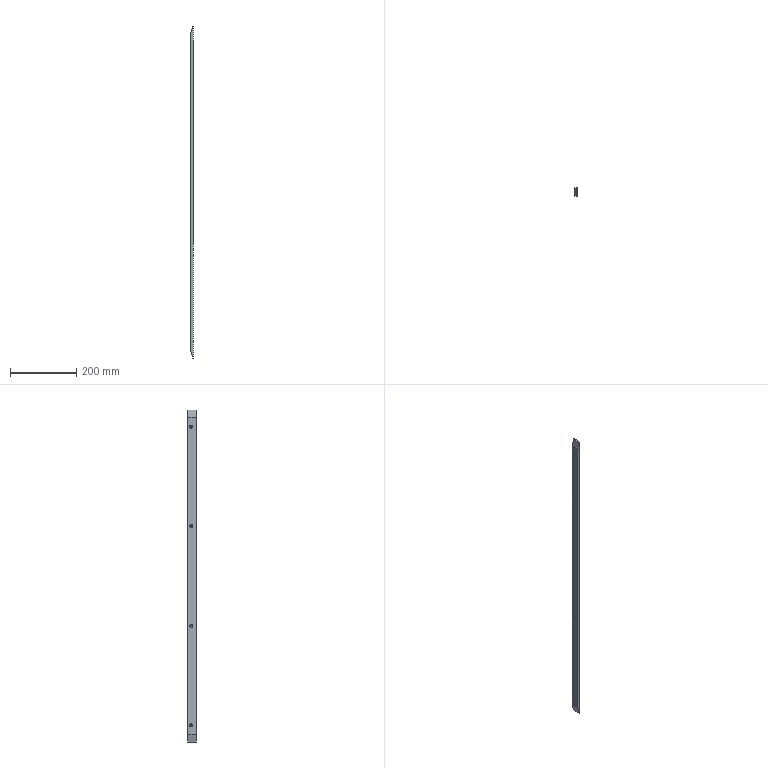Part | STEP file | 1 solid | 32 faces | box 8 x 25 x 1000 mm | volume 195560 mm3 | cylinder 16 | plane 8 | cone 8 | commonest cylinder face diameters 4.5 x8 9 x8